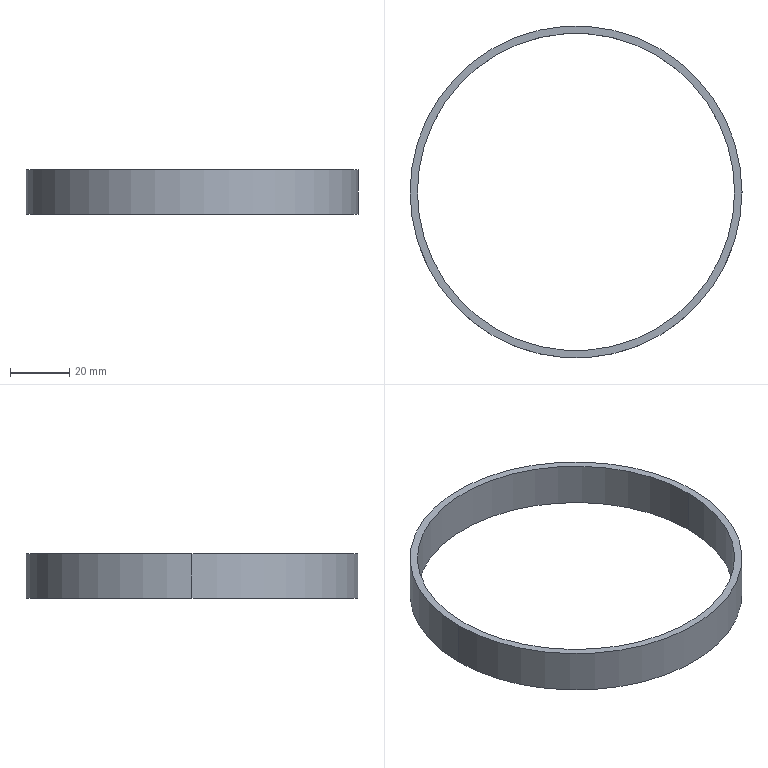Part | SolidWorks | features Extrusion 1 | 1 solid | 6 faces | box 112 x 112 x 15 mm | volume 12900 mm3 | cylinder 4 | plane 2 | commonest cylinder face diameters 107 x2 112 x2
STEP:
#1=CARTESIAN_POINT('',(-53.5,0.,15.));
#2=VERTEX_POINT('',#1);
#3=CARTESIAN_POINT('',(53.5,0.,15.));
#4=VERTEX_POINT('',#3);
#5=CARTESIAN_POINT('',(0.,0.,15.));
#6=DIRECTION('',(0.,0.,1.));
#7=DIRECTION('',(1.,0.,0.));
#8=AXIS2_PLACEMENT_3D('',#5,#6,#7);
#9=CIRCLE('',#8,53.5);
#10=EDGE_CURVE('',#2,#4,#9,.T.);
#11=ORIENTED_EDGE('',*,*,#10,.T.);
#12=CARTESIAN_POINT('',(53.5,0.,0.));
#13=VERTEX_POINT('',#12);
#14=CARTESIAN_POINT('',(53.5,0.,15.));
#15=DIRECTION('',(0.,0.,-1.));
#16=VECTOR('',#15,1000.);
#17=LINE('',#14,#16);
#18=EDGE_CURVE('',#4,#13,#17,.T.);
#19=ORIENTED_EDGE('',*,*,#18,.T.);
#20=CARTESIAN_POINT('',(-53.5,0.,0.));
#21=VERTEX_POINT('',#20);
#22=CARTESIAN_POINT('',(0.,0.,0.));
#23=DIRECTION('',(0.,0.,1.));
#24=DIRECTION('',(1.,0.,0.));
#25=AXIS2_PLACEMENT_3D('',#22,#23,#24);
#26=CIRCLE('',#25,53.5);
#27=EDGE_CURVE('',#21,#13,#26,.T.);
#28=ORIENTED_EDGE('',*,*,#27,.F.);
#29=CARTESIAN_POINT('',(-53.5,0.,15.));
#30=DIRECTION('',(0.,0.,-1.));
#31=VECTOR('',#30,1000.);
#32=LINE('',#29,#31);
#33=EDGE_CURVE('',#2,#21,#32,.T.);
#34=ORIENTED_EDGE('',*,*,#33,.F.);
#35=EDGE_LOOP('',(#11,#19,#28,#34));
#36=FACE_OUTER_BOUND('',#35,.T.);
#37=CARTESIAN_POINT('',(0.,0.,15.));
#38=DIRECTION('',(0.,0.,-1.));
#39=DIRECTION('',(-1.,0.,0.));
#40=AXIS2_PLACEMENT_3D('',#37,#38,#39);
#41=CYLINDRICAL_SURFACE('',#40,53.5);
#42=ADVANCED_FACE('',(#36),#41,.F.);
#43=CARTESIAN_POINT('',(56.,0.,15.));
#44=VERTEX_POINT('',#43);
#45=CARTESIAN_POINT('',(-56.,0.,15.));
#46=VERTEX_POINT('',#45);
#47=CARTESIAN_POINT('',(0.,0.,15.));
#48=DIRECTION('',(0.,0.,1.));
#49=DIRECTION('',(1.,0.,0.));
#50=AXIS2_PLACEMENT_3D('',#47,#48,#49);
#51=CIRCLE('',#50,56.);
#52=EDGE_CURVE('',#44,#46,#51,.T.);
#53=ORIENTED_EDGE('',*,*,#52,.F.);
#54=CARTESIAN_POINT('',(56.,0.,0.));
#55=VERTEX_POINT('',#54);
#56=CARTESIAN_POINT('',(56.,0.,15.));
#57=DIRECTION('',(0.,0.,-1.));
#58=VECTOR('',#57,1000.);
#59=LINE('',#56,#58);
#60=EDGE_CURVE('',#44,#55,#59,.T.);
#61=ORIENTED_EDGE('',*,*,#60,.T.);
#62=CARTESIAN_POINT('',(-56.,0.,0.));
#63=VERTEX_POINT('',#62);
#64=CARTESIAN_POINT('',(0.,0.,0.));
#65=DIRECTION('',(0.,0.,1.));
#66=DIRECTION('',(1.,0.,0.));
#67=AXIS2_PLACEMENT_3D('',#64,#65,#66);
#68=CIRCLE('',#67,56.);
#69=EDGE_CURVE('',#55,#63,#68,.T.);
#70=ORIENTED_EDGE('',*,*,#69,.T.);
#71=CARTESIAN_POINT('',(-56.,0.,15.));
#72=DIRECTION('',(0.,0.,-1.));
#73=VECTOR('',#72,1000.);
#74=LINE('',#71,#73);
#75=EDGE_CURVE('',#46,#63,#74,.T.);
#76=ORIENTED_EDGE('',*,*,#75,.F.);
#77=EDGE_LOOP('',(#53,#61,#70,#76));
#78=FACE_OUTER_BOUND('',#77,.T.);
#79=CARTESIAN_POINT('',(0.,0.,15.));
#80=DIRECTION('',(0.,0.,-1.));
#81=DIRECTION('',(-1.,0.,0.));
#82=AXIS2_PLACEMENT_3D('',#79,#80,#81);
#83=CYLINDRICAL_SURFACE('',#82,56.);
#84=ADVANCED_FACE('',(#78),#83,.T.);
#85=CARTESIAN_POINT('',(0.,0.,15.));
#86=DIRECTION('',(0.,0.,1.));
#87=DIRECTION('',(1.,0.,0.));
#88=AXIS2_PLACEMENT_3D('',#85,#86,#87);
#89=CIRCLE('',#88,56.);
#90=EDGE_CURVE('',#46,#44,#89,.T.);
#91=ORIENTED_EDGE('',*,*,#90,.T.);
#92=ORIENTED_EDGE('',*,*,#52,.T.);
#93=EDGE_LOOP('',(#91,#92));
#94=FACE_OUTER_BOUND('',#93,.T.);
#95=ORIENTED_EDGE('',*,*,#10,.F.);
#96=CARTESIAN_POINT('',(0.,0.,15.));
#97=DIRECTION('',(0.,0.,1.));
#98=DIRECTION('',(1.,0.,0.));
#99=AXIS2_PLACEMENT_3D('',#96,#97,#98);
#100=CIRCLE('',#99,53.5);
#101=EDGE_CURVE('',#4,#2,#100,.T.);
#102=ORIENTED_EDGE('',*,*,#101,.F.);
#103=EDGE_LOOP('',(#95,#102));
#104=FACE_BOUND('',#103,.T.);
#105=CARTESIAN_POINT('',(0.,0.,15.));
#106=DIRECTION('',(0.,0.,1.));
#107=DIRECTION('',(1.,0.,0.));
#108=AXIS2_PLACEMENT_3D('',#105,#106,#107);
#109=PLANE('',#108);
#110=ADVANCED_FACE('',(#94,#104),#109,.T.);
#111=CARTESIAN_POINT('',(0.,0.,0.));
#112=DIRECTION('',(0.,0.,1.));
#113=DIRECTION('',(1.,0.,0.));
#114=AXIS2_PLACEMENT_3D('',#111,#112,#113);
#115=CIRCLE('',#114,56.);
#116=EDGE_CURVE('',#63,#55,#115,.T.);
#117=ORIENTED_EDGE('',*,*,#116,.F.);
#118=ORIENTED_EDGE('',*,*,#69,.F.);
#119=EDGE_LOOP('',(#117,#118));
#120=FACE_OUTER_BOUND('',#119,.T.);
#121=ORIENTED_EDGE('',*,*,#27,.T.);
#122=CARTESIAN_POINT('',(0.,0.,0.));
#123=DIRECTION('',(0.,0.,1.));
#124=DIRECTION('',(1.,0.,0.));
#125=AXIS2_PLACEMENT_3D('',#122,#123,#124);
#126=CIRCLE('',#125,53.5);
#127=EDGE_CURVE('',#13,#21,#126,.T.);
#128=ORIENTED_EDGE('',*,*,#127,.T.);
#129=EDGE_LOOP('',(#121,#128));
#130=FACE_BOUND('',#129,.T.);
#131=CARTESIAN_POINT('',(0.,0.,0.));
#132=DIRECTION('',(0.,0.,1.));
#133=DIRECTION('',(1.,0.,0.));
#134=AXIS2_PLACEMENT_3D('',#131,#132,#133);
#135=PLANE('',#134);
#136=ADVANCED_FACE('',(#120,#130),#135,.F.);
#137=ORIENTED_EDGE('',*,*,#60,.F.);
#138=ORIENTED_EDGE('',*,*,#90,.F.);
#139=ORIENTED_EDGE('',*,*,#75,.T.);
#140=ORIENTED_EDGE('',*,*,#116,.T.);
#141=EDGE_LOOP('',(#137,#138,#139,#140));
#142=FACE_OUTER_BOUND('',#141,.T.);
#143=CARTESIAN_POINT('',(0.,0.,15.));
#144=DIRECTION('',(0.,0.,-1.));
#145=DIRECTION('',(-1.,0.,0.));
#146=AXIS2_PLACEMENT_3D('',#143,#144,#145);
#147=CYLINDRICAL_SURFACE('',#146,56.);
#148=ADVANCED_FACE('',(#142),#147,.T.);
#149=ORIENTED_EDGE('',*,*,#18,.F.);
#150=ORIENTED_EDGE('',*,*,#101,.T.);
#151=ORIENTED_EDGE('',*,*,#33,.T.);
#152=ORIENTED_EDGE('',*,*,#127,.F.);
#153=EDGE_LOOP('',(#149,#150,#151,#152));
#154=FACE_OUTER_BOUND('',#153,.T.);
#155=CARTESIAN_POINT('',(0.,0.,15.));
#156=DIRECTION('',(0.,0.,-1.));
#157=DIRECTION('',(-1.,0.,0.));
#158=AXIS2_PLACEMENT_3D('',#155,#156,#157);
#159=CYLINDRICAL_SURFACE('',#158,53.5);
#160=ADVANCED_FACE('',(#154),#159,.F.);
#161=CLOSED_SHELL('',(#42,#84,#110,#136,#148,#160));
#162=MANIFOLD_SOLID_BREP('',#161);
#163=CARTESIAN_POINT('',(0.,0.,0.));
#164=DIRECTION('',(0.,0.,1.));
#165=DIRECTION('',(1.,0.,0.));
#166=AXIS2_PLACEMENT_3D('',#163,#164,#165);
#167=(LENGTH_UNIT()NAMED_UNIT(*)SI_UNIT(.MILLI.,.METRE.));
#168=UNCERTAINTY_MEASURE_WITH_UNIT(LENGTH_MEASURE(0.00001),#167,'','');
#169=(NAMED_UNIT(*)PLANE_ANGLE_UNIT()SI_UNIT($,.RADIAN.));
#170=(NAMED_UNIT(*)SI_UNIT($,.STERADIAN.)SOLID_ANGLE_UNIT());
#171=(GEOMETRIC_REPRESENTATION_CONTEXT(3)GLOBAL_UNCERTAINTY_ASSIGNED_CONTEXT((#168))GLOBAL_UNIT_ASSIGNED_CONTEXT((#167,#169,#170))REPRESENTATION_CONTEXT('',''));
#172=ADVANCED_BREP_SHAPE_REPRESENTATION('',(#162,#166),#171);